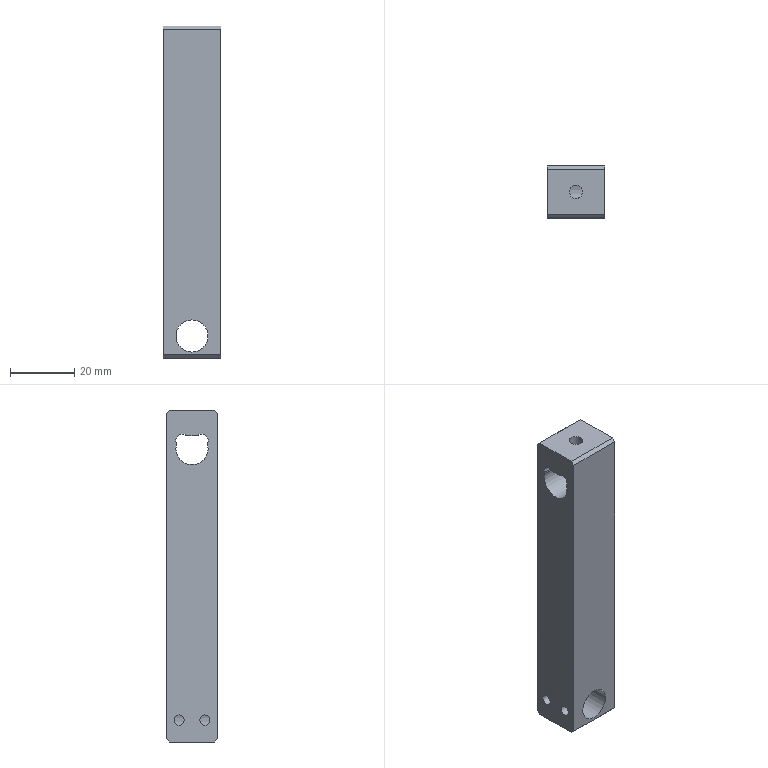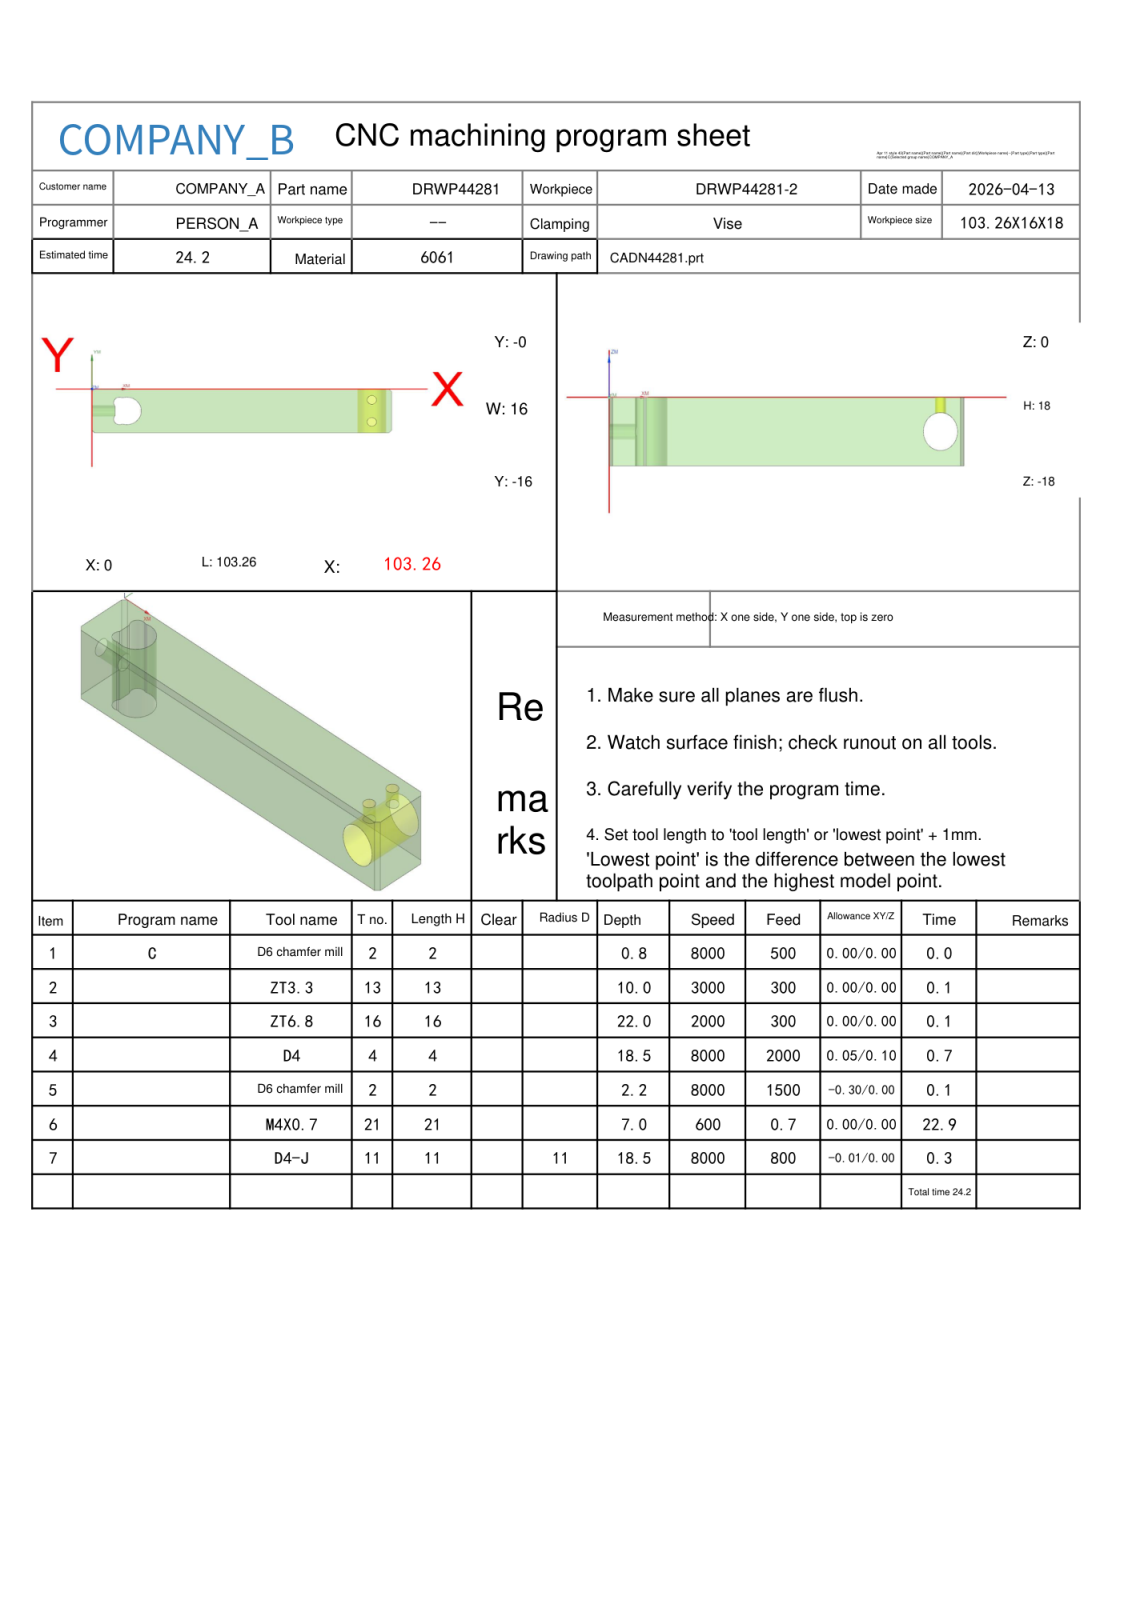NC program | NX | posted by the shop | part box 18 x 16 x 103.264 mm
Whole program:
%
O0001
(Machine time: 1.77 MIN)
(===Total Tool:2===)
(T1=D80R0.8 face mill D=80.  R=0.8  D-  H01 Z=0.    )
(T2=D6 chamfer mill   D=6.   R=0.   D-  H02 Z=-1.7  )
G80 G90 G17 G49 G40
G91 G28 Z0
M01
N1 T01 M06
(D80R0.8 face mill  D=80. R=0.8 H=01 ce=0.10 di=0.10)
G00 G90 G54 X-52.097 Y-9. M03 S5000
G43 H01 Z20.
M08
Z5.513
G01 Z3.513 F3000.
X-40.097
X143.361
X155.361
Z5.513
G00 X-52.097
Z5.025
G01 Z3.025
X-40.097
X143.361
X155.361
Z5.025
G00 X-52.097
Z4.538
G01 Z2.538
X-40.097
X143.361
X155.361
Z4.538
G00 X-52.097
Z4.05
G01 Z2.05
X-40.097
X143.361
X155.361
Z4.05
G00 Z20.
X-52.097
Z3.563
G01 Z1.563
X-40.097
X143.361
X155.361
Z3.563
G00 Z20.
X-52.097
Z3.075
G01 Z1.075
X-40.097
X143.361
X155.361
Z3.075
G00 Z20.
X-52.097
Z2.588
G01 Z.588
X-40.097
X143.361
X155.361
Z2.588
G00 Z20.
X-52.097
Z2.1
G01 Z.1
X-40.097
X143.361
X155.361
Z2.1
G00 Z20.
G91 G28 Z0.0
M05
M09
G91 G28 Z0.0
M01
N2 T01 M06
(D80R0.8 face mill-J  D=80. R=0.8 H=01 ce=0.00 di=0.00)
G00 G90 G54 X-51.999 Y-9. M03 S5000
G43 H01 Z20.
M08
Z2.
G01 Z0.0 F1000.
X-39.999
X143.263
X155.263
Z2.
G00 Z20.
G91 G28 Z0.0
M05
M09
G91 G28 Z0.0
M01
N3 T02 M06
(D6 chamfer mill  D=6. R=0. H=02 ce=0.00 di=0.00)
G00 G90 G54 X103.056 Y-18.99 M03 S6500
G43 H02 Z20.
M08
Z.13
G01 Z-1.2 F1500.
G03 X102.716 Y-18.915 I-.601 J-1.907
G01 X102.663 Y-18.905
X102.613 Y-18.928
X102.523 Y-18.966
X102.264 Y-19.
X1.
X.741 Y-18.966
X.651 Y-18.928
X.602 Y-18.905
X.548 Y-18.915
G03 X.208 Y-18.99 I.261 J-1.983
G01 Z.13
G00 Z10.
Y.99
Z.13
G01 Z-1.2
G03 X.548 Y.915 I.601 J1.907
G01 X.602 Y.905
X.651 Y.928
X.741 Y.966
X1. Y1.
X51.632
X102.264
X102.523 Y.966
X102.613 Y.928
X102.663 Y.905
X102.716 Y.915
G03 X103.056 Y.99 I-.261 J1.983
G01 Z.13
G00 Z2.55
X100.229 Y-9.4
Z.221
G01 Z-1.2
G03 X100.41 Y-9.102 I-1.613 J1.183
G01 X100.436 Y-9.054
X100.43 Y-9.
G03 X96.43 Y-5. I-4. J0.0
X92.43 Y-9. I0.0 J-4.
X96.43 Y-13. I4. J0.0
X100.43 Y-9. I0.0 J4.
G01 X100.436 Y-8.946
X100.41 Y-8.898
G03 X100.229 Y-8.6 I-1.794 J-.885
G01 Z.221
G00 Z20.
G00 G90 X-.885 Y-21.05 M03 S6500
Z20.
Z-.2
G01 Z-1.7 F1500.
G03 X-.85 Y-20.763 I-1.165 J.287
G01 Y2.763
G03 X-.885 Y3.05 I-1.2 J0.0
G01 Z-.2
G00 X-.735 Y-21.05
G01 Z-1.7
G03 X-.7 Y-20.763 I-1.165 J.287
G01 Y2.763
G03 X-.735 Y3.05 I-1.2 J0.0
G01 Z-.2
G00 Z20.
X104.149
Z-.2
G01 Z-1.7
G03 X104.114 Y2.763 I1.165 J-.287
G01 Y-20.763
G03 X104.149 Y-21.05 I1.2 J0.0
G01 Z-.2
G00 X103.999 Y3.05
G01 Z-1.7
G03 X103.964 Y2.763 I1.165 J-.287
G01 Y-20.763
G03 X103.999 Y-21.05 I1.2 J0.0
G01 Z-.2
G00 Z20.
M05
M09
G91 G28 Z0.0
G91 G28 Y0.0
M30
%